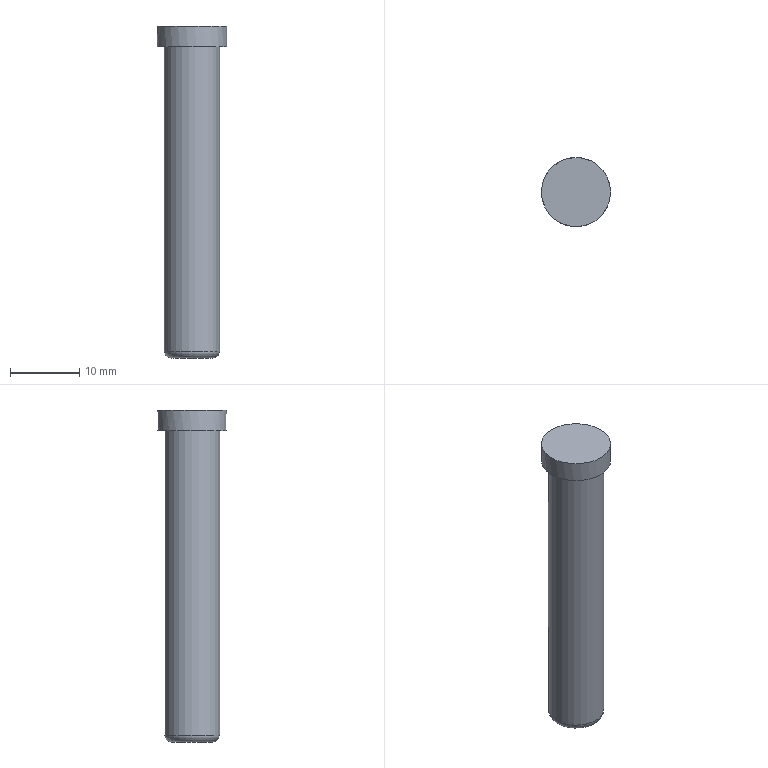Part | STEP file | gslz 2016.10.28-6_id334_x_t | 1 solid | 6 faces | box 10 x 10 x 48 mm | volume 2492 mm3 | plane 3 | cylinder 2 | torus 1 | commonest cylinder face diameters 8 x1 10 x1
STEP:
#1=CARTESIAN_POINT('',(-82.95,189.,111.492));
#2=VERTEX_POINT('',#1);
#3=CARTESIAN_POINT('',(-82.95,184.,111.492));
#4=DIRECTION('',(0.,0.,-1.));
#5=DIRECTION('',(0.,1.,0.));
#6=AXIS2_PLACEMENT_3D('',#3,#4,#5);
#7=CIRCLE('',#6,5.);
#8=EDGE_CURVE('',#2,#2,#7,.T.);
#9=ORIENTED_EDGE('',*,*,#8,.F.);
#10=EDGE_LOOP('',(#9));
#11=FACE_OUTER_BOUND('',#10,.T.);
#12=CARTESIAN_POINT('',(-27.511,228.829,111.492));
#13=DIRECTION('',(0.,0.,1.));
#14=DIRECTION('',(-1.,0.,0.));
#15=AXIS2_PLACEMENT_3D('',#12,#13,#14);
#16=PLANE('',#15);
#17=ADVANCED_FACE('',(#11),#16,.T.);
#18=CARTESIAN_POINT('',(-78.95,184.,108.492));
#19=VERTEX_POINT('',#18);
#20=CARTESIAN_POINT('',(-82.95,184.,108.492));
#21=DIRECTION('',(0.,0.,-1.));
#22=DIRECTION('',(1.,0.,0.));
#23=AXIS2_PLACEMENT_3D('',#20,#21,#22);
#24=CIRCLE('',#23,4.);
#25=EDGE_CURVE('',#19,#19,#24,.T.);
#26=ORIENTED_EDGE('',*,*,#25,.F.);
#27=EDGE_LOOP('',(#26));
#28=FACE_BOUND('',#27,.T.);
#29=CARTESIAN_POINT('',(-77.95,184.,108.492));
#30=VERTEX_POINT('',#29);
#31=CARTESIAN_POINT('',(-82.95,184.,108.492));
#32=DIRECTION('',(0.,0.,1.));
#33=DIRECTION('',(1.,0.,0.));
#34=AXIS2_PLACEMENT_3D('',#31,#32,#33);
#35=CIRCLE('',#34,5.);
#36=EDGE_CURVE('',#30,#30,#35,.T.);
#37=ORIENTED_EDGE('',*,*,#36,.F.);
#38=EDGE_LOOP('',(#37));
#39=FACE_BOUND('',#38,.T.);
#40=CARTESIAN_POINT('',(-82.95,184.,108.492));
#41=DIRECTION('',(0.,0.,-1.));
#42=DIRECTION('',(1.,0.,0.));
#43=AXIS2_PLACEMENT_3D('',#40,#41,#42);
#44=PLANE('',#43);
#45=ADVANCED_FACE('',(#28,#39),#44,.T.);
#46=ORIENTED_EDGE('',*,*,#8,.T.);
#47=EDGE_LOOP('',(#46));
#48=FACE_BOUND('',#47,.T.);
#49=ORIENTED_EDGE('',*,*,#36,.T.);
#50=EDGE_LOOP('',(#49));
#51=FACE_BOUND('',#50,.T.);
#52=CARTESIAN_POINT('',(-82.95,184.,90.492));
#53=DIRECTION('',(0.,0.,1.));
#54=DIRECTION('',(1.,0.,0.));
#55=AXIS2_PLACEMENT_3D('',#52,#53,#54);
#56=CYLINDRICAL_SURFACE('',#55,5.);
#57=ADVANCED_FACE('',(#48,#51),#56,.T.);
#58=CARTESIAN_POINT('',(-79.95,184.,63.492));
#59=VERTEX_POINT('',#58);
#60=CARTESIAN_POINT('',(-82.95,184.,63.492));
#61=DIRECTION('',(0.,0.,1.));
#62=DIRECTION('',(1.,0.,0.));
#63=AXIS2_PLACEMENT_3D('',#60,#61,#62);
#64=CIRCLE('',#63,3.);
#65=EDGE_CURVE('',#59,#59,#64,.T.);
#66=ORIENTED_EDGE('',*,*,#65,.F.);
#67=EDGE_LOOP('',(#66));
#68=FACE_OUTER_BOUND('',#67,.T.);
#69=CARTESIAN_POINT('',(-82.95,184.,63.492));
#70=DIRECTION('',(0.,0.,-1.));
#71=DIRECTION('',(-1.,0.,0.));
#72=AXIS2_PLACEMENT_3D('',#69,#70,#71);
#73=PLANE('',#72);
#74=ADVANCED_FACE('',(#68),#73,.T.);
#75=CARTESIAN_POINT('',(-78.95,184.,64.492));
#76=VERTEX_POINT('',#75);
#77=CARTESIAN_POINT('',(-82.95,184.,64.492));
#78=DIRECTION('',(0.,0.,-1.));
#79=DIRECTION('',(1.,0.,0.));
#80=AXIS2_PLACEMENT_3D('',#77,#78,#79);
#81=CIRCLE('',#80,4.);
#82=EDGE_CURVE('',#76,#76,#81,.T.);
#83=ORIENTED_EDGE('',*,*,#82,.F.);
#84=EDGE_LOOP('',(#83));
#85=FACE_BOUND('',#84,.T.);
#86=ORIENTED_EDGE('',*,*,#25,.T.);
#87=EDGE_LOOP('',(#86));
#88=FACE_BOUND('',#87,.T.);
#89=CARTESIAN_POINT('',(-82.95,184.,100.492));
#90=DIRECTION('',(0.,0.,-1.));
#91=DIRECTION('',(-1.,0.,0.));
#92=AXIS2_PLACEMENT_3D('',#89,#90,#91);
#93=CYLINDRICAL_SURFACE('',#92,4.);
#94=ADVANCED_FACE('',(#85,#88),#93,.T.);
#95=ORIENTED_EDGE('',*,*,#82,.T.);
#96=EDGE_LOOP('',(#95));
#97=FACE_BOUND('',#96,.T.);
#98=ORIENTED_EDGE('',*,*,#65,.T.);
#99=EDGE_LOOP('',(#98));
#100=FACE_BOUND('',#99,.T.);
#101=CARTESIAN_POINT('',(-82.95,184.,64.492));
#102=DIRECTION('',(0.,0.,-1.));
#103=DIRECTION('',(-1.,0.,0.));
#104=AXIS2_PLACEMENT_3D('',#101,#102,#103);
#105=TOROIDAL_SURFACE('',#104,3.,1.);
#106=ADVANCED_FACE('',(#97,#100),#105,.T.);
#107=CLOSED_SHELL('',(#17,#45,#57,#74,#94,#106));
#108=MANIFOLD_SOLID_BREP('',#107);
#109=(LENGTH_UNIT()NAMED_UNIT(*)SI_UNIT(.MILLI.,.METRE.));
#110=UNCERTAINTY_MEASURE_WITH_UNIT(LENGTH_MEASURE(0.00002),#109,'','');
#111=(NAMED_UNIT(*)PLANE_ANGLE_UNIT()SI_UNIT($,.RADIAN.));
#112=PLANE_ANGLE_MEASURE_WITH_UNIT(PLANE_ANGLE_MEASURE(0.01745),#111);
#113=DIMENSIONAL_EXPONENTS(0.,0.,0.,0.,0.,0.,0.);
#114=(CONVERSION_BASED_UNIT('DEGREE',#112)NAMED_UNIT(#113)PLANE_ANGLE_UNIT());
#115=(NAMED_UNIT(*)SI_UNIT($,.STERADIAN.)SOLID_ANGLE_UNIT());
#116=(GEOMETRIC_REPRESENTATION_CONTEXT(3)GLOBAL_UNCERTAINTY_ASSIGNED_CONTEXT((#110))GLOBAL_UNIT_ASSIGNED_CONTEXT((#109,#114,#115))REPRESENTATION_CONTEXT('',''));
#117=ADVANCED_BREP_SHAPE_REPRESENTATION('',(#108),#116);